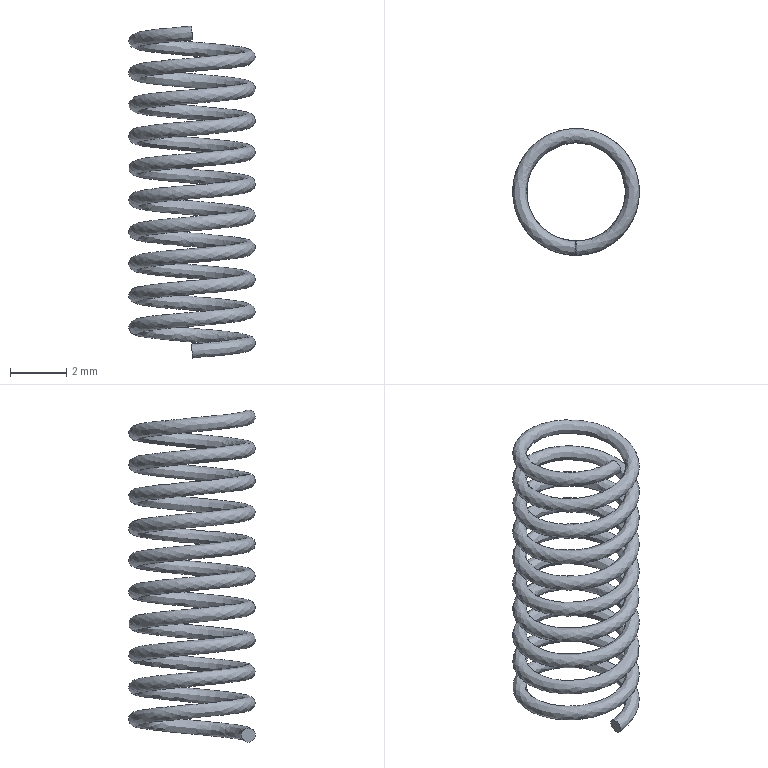Part | STEP file | 1-16.3 | 1 solid | 3 faces | box 4.501 x 4.5 x 11.798 mm | volume 24.723 mm3 | plane 2 | spline 1